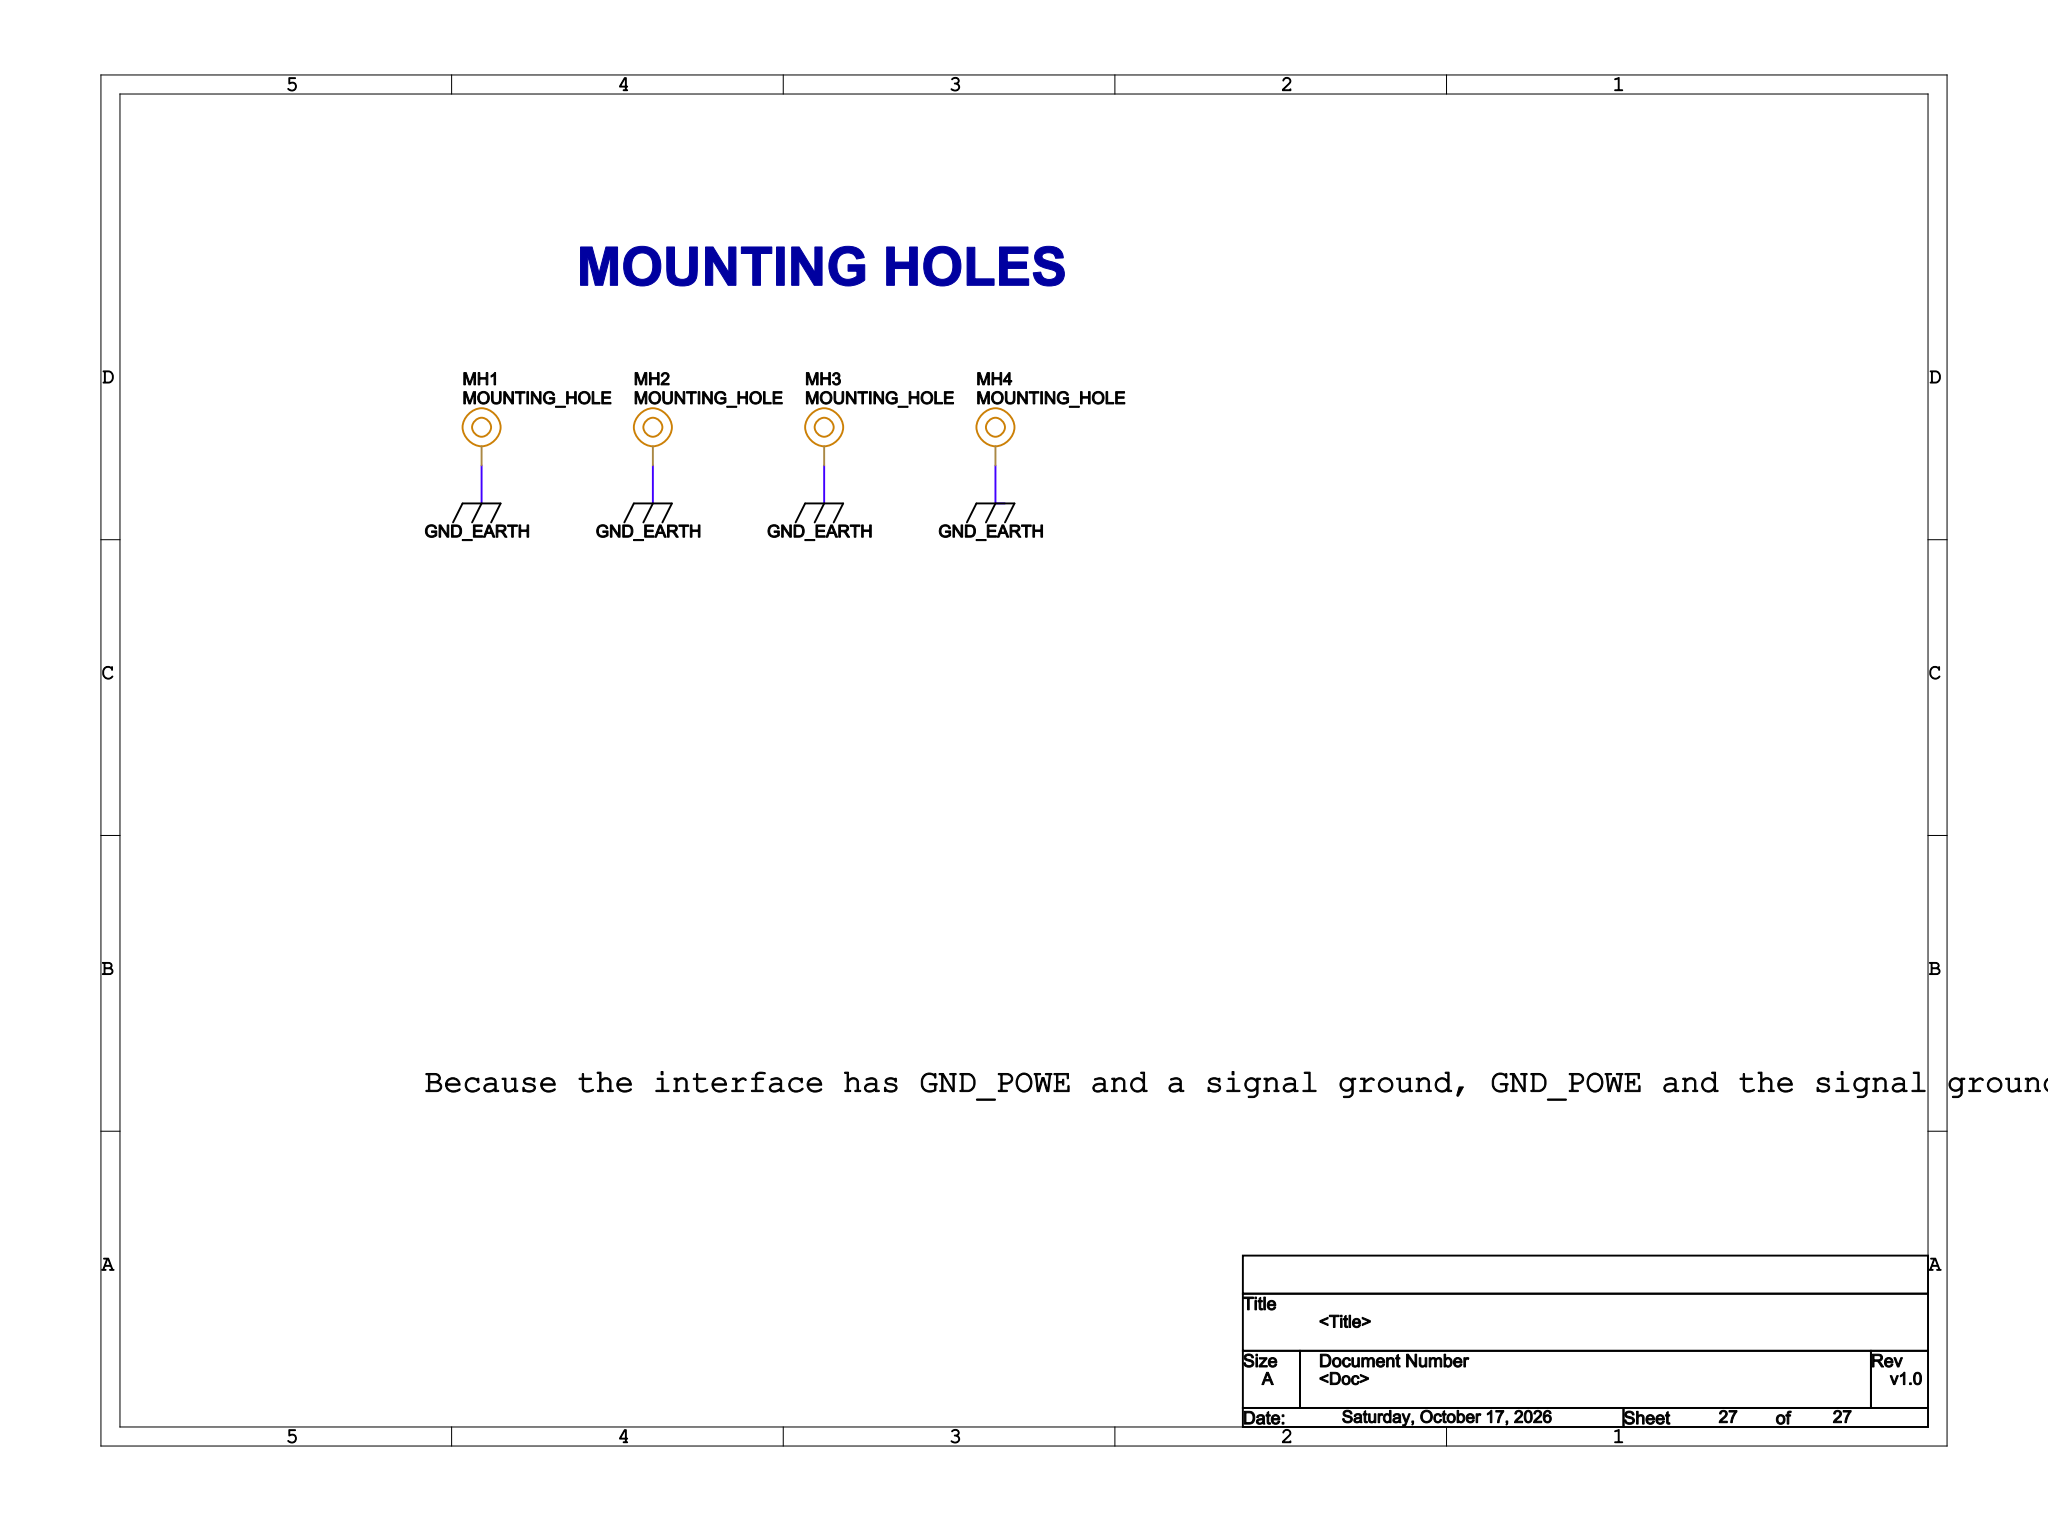Circuit board | Cadence Allegro | 477 parts | 327 nets | one sheet of the schematic
Parts on this sheet (reference | value | footprint):
MH1 | MOUNTING_HOLE | HOLE2_2_4
MH2 | MOUNTING_HOLE | HOLE2_2_4
MH3 | MOUNTING_HOLE | HOLE2_2_4
MH4 | MOUNTING_HOLE | HOLE2_2_4
Nets of these parts (net: part-pin ...):
GND_EARTH: MH1-1 MH2-1 MH3-1 MH4-1